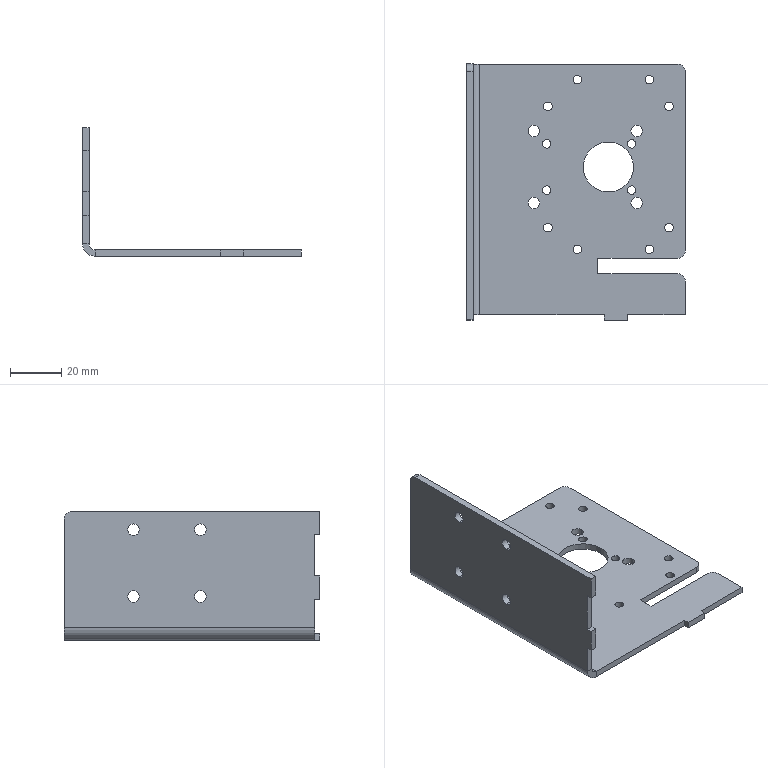Part | SolidWorks | features Cut 4, Fillet 2, ICE 2, EdgeFlange 1, FlatPattern 1, LPattern 1, SMBaseFlange 1, SheetMetal 1 | 1 solid | 74 faces | box 85 x 99.5 x 50 mm | volume 30184 mm3 | cylinder 48 | plane 26 | commonest cylinder face diameters 3.3 x16 4.5 x16 3.4 x8 6 x4 19.5 x2 5 x1